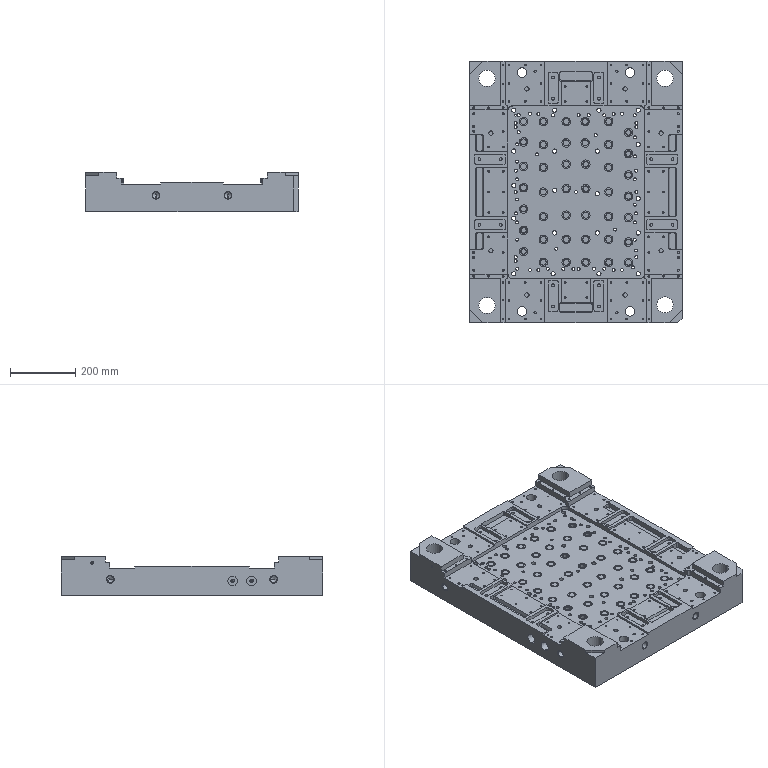Part | Creo | 1 solid | 1558 faces | box 650 x 800 x 120 mm | volume 40896959 mm3 | cylinder 927 | plane 350 | cone 281 | commonest cylinder face diameters 5 x200 9 x108 18 x84 26 x84 10 x74 13 x56